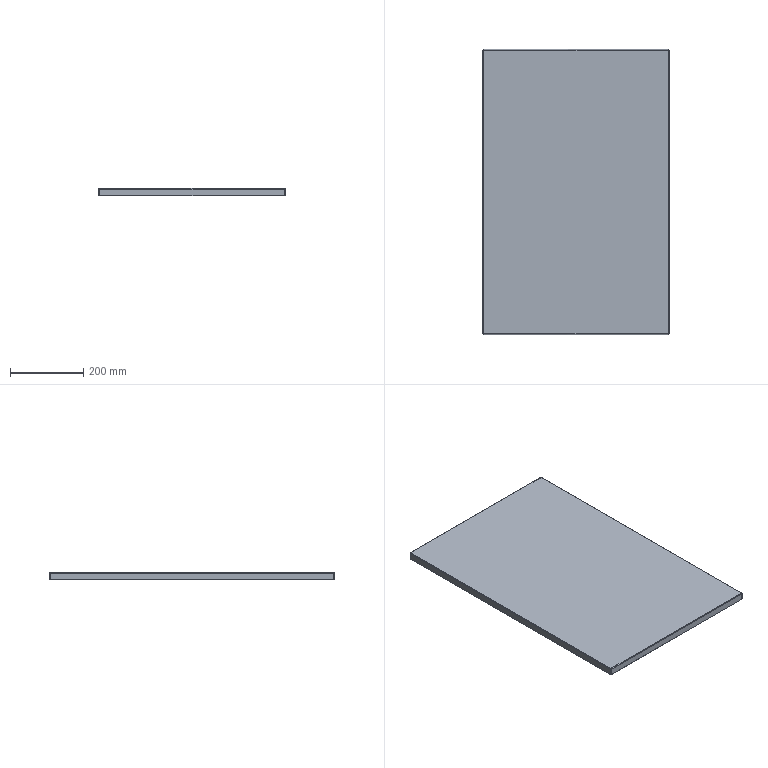Part | STEP file | X77-03013 | 1 solid | 38 faces | box 508 x 778 x 20 mm | volume 661245 mm3 | plane 22 | spline 8 | cylinder 8 | commonest cylinder face diameters 1.473 x4 4.473 x4